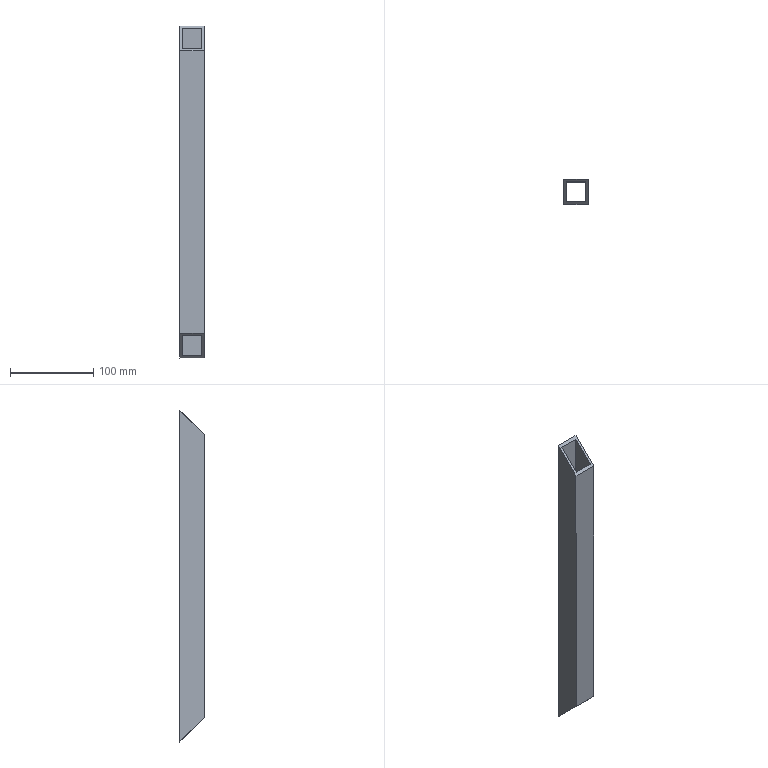Part | SolidWorks | features ICE 3, Extrusion 1 | 1 solid | 10 faces | box 30 x 30 x 400 mm | volume 119880 mm3 | plane 10
STEP:
#1=CARTESIAN_POINT('',(-45.142,-4.099,370.));
#2=VERTEX_POINT('',#1);
#3=CARTESIAN_POINT('',(-45.142,-4.099,30.));
#4=VERTEX_POINT('',#3);
#5=CARTESIAN_POINT('',(-45.142,-4.099,400.));
#6=DIRECTION('',(0.,0.,-1.));
#7=VECTOR('',#6,1000.);
#8=LINE('',#5,#7);
#9=EDGE_CURVE('',#2,#4,#8,.T.);
#10=ORIENTED_EDGE('',*,*,#9,.F.);
#11=CARTESIAN_POINT('',(-45.142,25.901,400.));
#12=VERTEX_POINT('',#11);
#13=CARTESIAN_POINT('',(-45.142,25.901,400.));
#14=DIRECTION('',(0.,0.7071,0.7071));
#15=VECTOR('',#14,1000.);
#16=LINE('',#13,#15);
#17=EDGE_CURVE('',#2,#12,#16,.T.);
#18=ORIENTED_EDGE('',*,*,#17,.T.);
#19=CARTESIAN_POINT('',(-45.142,25.901,0.));
#20=VERTEX_POINT('',#19);
#21=CARTESIAN_POINT('',(-45.142,25.901,400.));
#22=DIRECTION('',(0.,0.,-1.));
#23=VECTOR('',#22,1000.);
#24=LINE('',#21,#23);
#25=EDGE_CURVE('',#12,#20,#24,.T.);
#26=ORIENTED_EDGE('',*,*,#25,.T.);
#27=CARTESIAN_POINT('',(-45.142,25.901,0.));
#28=DIRECTION('',(0.,-0.7071,0.7071));
#29=VECTOR('',#28,1000.);
#30=LINE('',#27,#29);
#31=EDGE_CURVE('',#20,#4,#30,.T.);
#32=ORIENTED_EDGE('',*,*,#31,.T.);
#33=EDGE_LOOP('',(#10,#18,#26,#32));
#34=FACE_OUTER_BOUND('',#33,.T.);
#35=CARTESIAN_POINT('',(-45.142,-4.099,400.));
#36=DIRECTION('',(1.,0.,0.));
#37=DIRECTION('',(0.,0.,-1.));
#38=AXIS2_PLACEMENT_3D('',#35,#36,#37);
#39=PLANE('',#38);
#40=ADVANCED_FACE('',(#34),#39,.F.);
#41=CARTESIAN_POINT('',(-15.142,-4.099,370.));
#42=VERTEX_POINT('',#41);
#43=CARTESIAN_POINT('',(-15.142,-4.099,30.));
#44=VERTEX_POINT('',#43);
#45=CARTESIAN_POINT('',(-15.142,-4.099,400.));
#46=DIRECTION('',(0.,0.,-1.));
#47=VECTOR('',#46,1000.);
#48=LINE('',#45,#47);
#49=EDGE_CURVE('',#42,#44,#48,.T.);
#50=ORIENTED_EDGE('',*,*,#49,.F.);
#51=CARTESIAN_POINT('',(-45.142,-4.099,370.));
#52=DIRECTION('',(1.,0.,0.));
#53=VECTOR('',#52,1000.);
#54=LINE('',#51,#53);
#55=EDGE_CURVE('',#2,#42,#54,.T.);
#56=ORIENTED_EDGE('',*,*,#55,.F.);
#57=ORIENTED_EDGE('',*,*,#9,.T.);
#58=CARTESIAN_POINT('',(-45.142,-4.099,30.));
#59=DIRECTION('',(1.,0.,0.));
#60=VECTOR('',#59,1000.);
#61=LINE('',#58,#60);
#62=EDGE_CURVE('',#4,#44,#61,.T.);
#63=ORIENTED_EDGE('',*,*,#62,.T.);
#64=EDGE_LOOP('',(#50,#56,#57,#63));
#65=FACE_OUTER_BOUND('',#64,.T.);
#66=CARTESIAN_POINT('',(-15.142,-4.099,400.));
#67=DIRECTION('',(0.,1.,0.));
#68=DIRECTION('',(0.,0.,1.));
#69=AXIS2_PLACEMENT_3D('',#66,#67,#68);
#70=PLANE('',#69);
#71=ADVANCED_FACE('',(#65),#70,.F.);
#72=CARTESIAN_POINT('',(-15.142,25.901,400.));
#73=VERTEX_POINT('',#72);
#74=CARTESIAN_POINT('',(-15.142,25.901,0.));
#75=VERTEX_POINT('',#74);
#76=CARTESIAN_POINT('',(-15.142,25.901,400.));
#77=DIRECTION('',(0.,0.,-1.));
#78=VECTOR('',#77,1000.);
#79=LINE('',#76,#78);
#80=EDGE_CURVE('',#73,#75,#79,.T.);
#81=ORIENTED_EDGE('',*,*,#80,.F.);
#82=CARTESIAN_POINT('',(-15.142,25.901,400.));
#83=DIRECTION('',(0.,0.7071,0.7071));
#84=VECTOR('',#83,1000.);
#85=LINE('',#82,#84);
#86=EDGE_CURVE('',#42,#73,#85,.T.);
#87=ORIENTED_EDGE('',*,*,#86,.F.);
#88=ORIENTED_EDGE('',*,*,#49,.T.);
#89=CARTESIAN_POINT('',(-15.142,25.901,0.));
#90=DIRECTION('',(0.,-0.7071,0.7071));
#91=VECTOR('',#90,1000.);
#92=LINE('',#89,#91);
#93=EDGE_CURVE('',#75,#44,#92,.T.);
#94=ORIENTED_EDGE('',*,*,#93,.F.);
#95=EDGE_LOOP('',(#81,#87,#88,#94));
#96=FACE_OUTER_BOUND('',#95,.T.);
#97=CARTESIAN_POINT('',(-15.142,25.901,400.));
#98=DIRECTION('',(-1.,0.,0.));
#99=DIRECTION('',(0.,0.,1.));
#100=AXIS2_PLACEMENT_3D('',#97,#98,#99);
#101=PLANE('',#100);
#102=ADVANCED_FACE('',(#96),#101,.F.);
#103=CARTESIAN_POINT('',(-45.142,25.901,0.));
#104=DIRECTION('',(-1.,0.,0.));
#105=VECTOR('',#104,1000.);
#106=LINE('',#103,#105);
#107=EDGE_CURVE('',#75,#20,#106,.T.);
#108=ORIENTED_EDGE('',*,*,#107,.T.);
#109=ORIENTED_EDGE('',*,*,#25,.F.);
#110=CARTESIAN_POINT('',(-45.142,25.901,400.));
#111=DIRECTION('',(-1.,0.,0.));
#112=VECTOR('',#111,1000.);
#113=LINE('',#110,#112);
#114=EDGE_CURVE('',#73,#12,#113,.T.);
#115=ORIENTED_EDGE('',*,*,#114,.F.);
#116=ORIENTED_EDGE('',*,*,#80,.T.);
#117=EDGE_LOOP('',(#108,#109,#115,#116));
#118=FACE_OUTER_BOUND('',#117,.T.);
#119=CARTESIAN_POINT('',(-45.142,25.901,400.));
#120=DIRECTION('',(0.,-1.,0.));
#121=DIRECTION('',(0.,0.,-1.));
#122=AXIS2_PLACEMENT_3D('',#119,#120,#121);
#123=PLANE('',#122);
#124=ADVANCED_FACE('',(#118),#123,.F.);
#125=CARTESIAN_POINT('',(-42.142,22.901,3.));
#126=VERTEX_POINT('',#125);
#127=CARTESIAN_POINT('',(-42.142,22.901,397.));
#128=VERTEX_POINT('',#127);
#129=CARTESIAN_POINT('',(-42.142,22.901,-92.));
#130=DIRECTION('',(0.,0.,1.));
#131=VECTOR('',#130,1000.);
#132=LINE('',#129,#131);
#133=EDGE_CURVE('',#126,#128,#132,.T.);
#134=ORIENTED_EDGE('',*,*,#133,.T.);
#135=CARTESIAN_POINT('',(-42.142,-1.099,373.));
#136=VERTEX_POINT('',#135);
#137=CARTESIAN_POINT('',(-42.142,-233.599,140.5));
#138=DIRECTION('',(0.,-0.7071,-0.7071));
#139=VECTOR('',#138,1000.);
#140=LINE('',#137,#139);
#141=EDGE_CURVE('',#128,#136,#140,.T.);
#142=ORIENTED_EDGE('',*,*,#141,.T.);
#143=CARTESIAN_POINT('',(-42.142,-1.099,27.));
#144=VERTEX_POINT('',#143);
#145=CARTESIAN_POINT('',(-42.142,-1.099,-92.));
#146=DIRECTION('',(0.,0.,1.));
#147=VECTOR('',#146,1000.);
#148=LINE('',#145,#147);
#149=EDGE_CURVE('',#144,#136,#148,.T.);
#150=ORIENTED_EDGE('',*,*,#149,.F.);
#151=CARTESIAN_POINT('',(-42.142,58.401,-32.5));
#152=DIRECTION('',(0.,0.7071,-0.7071));
#153=VECTOR('',#152,1000.);
#154=LINE('',#151,#153);
#155=EDGE_CURVE('',#144,#126,#154,.T.);
#156=ORIENTED_EDGE('',*,*,#155,.T.);
#157=EDGE_LOOP('',(#134,#142,#150,#156));
#158=FACE_OUTER_BOUND('',#157,.T.);
#159=CARTESIAN_POINT('',(-42.142,-1.099,-92.));
#160=DIRECTION('',(-1.,0.,0.));
#161=DIRECTION('',(0.,0.,1.));
#162=AXIS2_PLACEMENT_3D('',#159,#160,#161);
#163=PLANE('',#162);
#164=ADVANCED_FACE('',(#158),#163,.F.);
#165=CARTESIAN_POINT('',(-18.142,22.901,3.));
#166=VERTEX_POINT('',#165);
#167=CARTESIAN_POINT('',(-18.142,22.901,397.));
#168=VERTEX_POINT('',#167);
#169=CARTESIAN_POINT('',(-18.142,22.901,-92.));
#170=DIRECTION('',(0.,0.,1.));
#171=VECTOR('',#170,1000.);
#172=LINE('',#169,#171);
#173=EDGE_CURVE('',#166,#168,#172,.T.);
#174=ORIENTED_EDGE('',*,*,#173,.T.);
#175=CARTESIAN_POINT('',(-42.142,22.901,397.));
#176=DIRECTION('',(-1.,0.,0.));
#177=VECTOR('',#176,1000.);
#178=LINE('',#175,#177);
#179=EDGE_CURVE('',#168,#128,#178,.T.);
#180=ORIENTED_EDGE('',*,*,#179,.T.);
#181=ORIENTED_EDGE('',*,*,#133,.F.);
#182=CARTESIAN_POINT('',(-42.142,22.901,3.));
#183=DIRECTION('',(1.,0.,0.));
#184=VECTOR('',#183,1000.);
#185=LINE('',#182,#184);
#186=EDGE_CURVE('',#126,#166,#185,.T.);
#187=ORIENTED_EDGE('',*,*,#186,.T.);
#188=EDGE_LOOP('',(#174,#180,#181,#187));
#189=FACE_OUTER_BOUND('',#188,.T.);
#190=CARTESIAN_POINT('',(-42.142,22.901,-92.));
#191=DIRECTION('',(0.,1.,0.));
#192=DIRECTION('',(0.,0.,1.));
#193=AXIS2_PLACEMENT_3D('',#190,#191,#192);
#194=PLANE('',#193);
#195=ADVANCED_FACE('',(#189),#194,.F.);
#196=CARTESIAN_POINT('',(-18.142,-1.099,27.));
#197=VERTEX_POINT('',#196);
#198=CARTESIAN_POINT('',(-18.142,-1.099,373.));
#199=VERTEX_POINT('',#198);
#200=CARTESIAN_POINT('',(-18.142,-1.099,-92.));
#201=DIRECTION('',(0.,0.,1.));
#202=VECTOR('',#201,1000.);
#203=LINE('',#200,#202);
#204=EDGE_CURVE('',#197,#199,#203,.T.);
#205=ORIENTED_EDGE('',*,*,#204,.T.);
#206=CARTESIAN_POINT('',(-18.142,-221.599,152.5));
#207=DIRECTION('',(0.,0.7071,0.7071));
#208=VECTOR('',#207,1000.);
#209=LINE('',#206,#208);
#210=EDGE_CURVE('',#199,#168,#209,.T.);
#211=ORIENTED_EDGE('',*,*,#210,.T.);
#212=ORIENTED_EDGE('',*,*,#173,.F.);
#213=CARTESIAN_POINT('',(-18.142,70.401,-44.5));
#214=DIRECTION('',(0.,-0.7071,0.7071));
#215=VECTOR('',#214,1000.);
#216=LINE('',#213,#215);
#217=EDGE_CURVE('',#166,#197,#216,.T.);
#218=ORIENTED_EDGE('',*,*,#217,.T.);
#219=EDGE_LOOP('',(#205,#211,#212,#218));
#220=FACE_OUTER_BOUND('',#219,.T.);
#221=CARTESIAN_POINT('',(-18.142,22.901,-92.));
#222=DIRECTION('',(1.,0.,0.));
#223=DIRECTION('',(0.,1.,0.));
#224=AXIS2_PLACEMENT_3D('',#221,#222,#223);
#225=PLANE('',#224);
#226=ADVANCED_FACE('',(#220),#225,.F.);
#227=ORIENTED_EDGE('',*,*,#149,.T.);
#228=CARTESIAN_POINT('',(-18.142,-1.099,373.));
#229=DIRECTION('',(1.,0.,0.));
#230=VECTOR('',#229,1000.);
#231=LINE('',#228,#230);
#232=EDGE_CURVE('',#136,#199,#231,.T.);
#233=ORIENTED_EDGE('',*,*,#232,.T.);
#234=ORIENTED_EDGE('',*,*,#204,.F.);
#235=CARTESIAN_POINT('',(-18.142,-1.099,27.));
#236=DIRECTION('',(-1.,0.,0.));
#237=VECTOR('',#236,1000.);
#238=LINE('',#235,#237);
#239=EDGE_CURVE('',#197,#144,#238,.T.);
#240=ORIENTED_EDGE('',*,*,#239,.T.);
#241=EDGE_LOOP('',(#227,#233,#234,#240));
#242=FACE_OUTER_BOUND('',#241,.T.);
#243=CARTESIAN_POINT('',(-18.142,-1.099,-92.));
#244=DIRECTION('',(0.,-1.,0.));
#245=DIRECTION('',(1.,0.,0.));
#246=AXIS2_PLACEMENT_3D('',#243,#244,#245);
#247=PLANE('',#246);
#248=ADVANCED_FACE('',(#242),#247,.F.);
#249=ORIENTED_EDGE('',*,*,#93,.T.);
#250=ORIENTED_EDGE('',*,*,#62,.F.);
#251=ORIENTED_EDGE('',*,*,#31,.F.);
#252=ORIENTED_EDGE('',*,*,#107,.F.);
#253=EDGE_LOOP('',(#249,#250,#251,#252));
#254=FACE_OUTER_BOUND('',#253,.T.);
#255=ORIENTED_EDGE('',*,*,#239,.F.);
#256=ORIENTED_EDGE('',*,*,#217,.F.);
#257=ORIENTED_EDGE('',*,*,#186,.F.);
#258=ORIENTED_EDGE('',*,*,#155,.F.);
#259=EDGE_LOOP('',(#255,#256,#257,#258));
#260=FACE_BOUND('',#259,.T.);
#261=CARTESIAN_POINT('',(-45.142,25.901,0.));
#262=DIRECTION('',(0.,0.7071,0.7071));
#263=DIRECTION('',(0.,-0.7071,0.7071));
#264=AXIS2_PLACEMENT_3D('',#261,#262,#263);
#265=PLANE('',#264);
#266=ADVANCED_FACE('',(#254,#260),#265,.F.);
#267=ORIENTED_EDGE('',*,*,#86,.T.);
#268=ORIENTED_EDGE('',*,*,#114,.T.);
#269=ORIENTED_EDGE('',*,*,#17,.F.);
#270=ORIENTED_EDGE('',*,*,#55,.T.);
#271=EDGE_LOOP('',(#267,#268,#269,#270));
#272=FACE_OUTER_BOUND('',#271,.T.);
#273=ORIENTED_EDGE('',*,*,#179,.F.);
#274=ORIENTED_EDGE('',*,*,#210,.F.);
#275=ORIENTED_EDGE('',*,*,#232,.F.);
#276=ORIENTED_EDGE('',*,*,#141,.F.);
#277=EDGE_LOOP('',(#273,#274,#275,#276));
#278=FACE_BOUND('',#277,.T.);
#279=CARTESIAN_POINT('',(-45.142,25.901,400.));
#280=DIRECTION('',(0.,0.7071,-0.7071));
#281=DIRECTION('',(0.,0.7071,0.7071));
#282=AXIS2_PLACEMENT_3D('',#279,#280,#281);
#283=PLANE('',#282);
#284=ADVANCED_FACE('',(#272,#278),#283,.F.);
#285=CLOSED_SHELL('',(#40,#71,#102,#124,#164,#195,#226,#248,#266,#284));
#286=MANIFOLD_SOLID_BREP('',#285);
#287=CARTESIAN_POINT('',(0.,0.,0.));
#288=DIRECTION('',(0.,0.,1.));
#289=DIRECTION('',(1.,0.,0.));
#290=AXIS2_PLACEMENT_3D('',#287,#288,#289);
#291=(LENGTH_UNIT()NAMED_UNIT(*)SI_UNIT(.MILLI.,.METRE.));
#292=UNCERTAINTY_MEASURE_WITH_UNIT(LENGTH_MEASURE(0.00001),#291,'','');
#293=(NAMED_UNIT(*)PLANE_ANGLE_UNIT()SI_UNIT($,.RADIAN.));
#294=(NAMED_UNIT(*)SI_UNIT($,.STERADIAN.)SOLID_ANGLE_UNIT());
#295=(GEOMETRIC_REPRESENTATION_CONTEXT(3)GLOBAL_UNCERTAINTY_ASSIGNED_CONTEXT((#292))GLOBAL_UNIT_ASSIGNED_CONTEXT((#291,#293,#294))REPRESENTATION_CONTEXT('',''));
#296=ADVANCED_BREP_SHAPE_REPRESENTATION('',(#286,#290),#295);